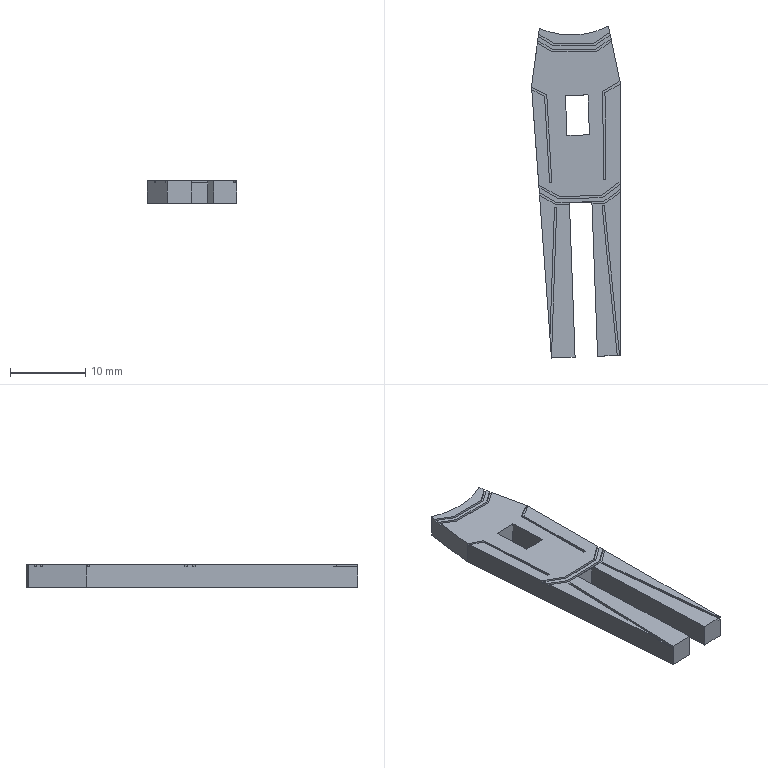Part | SolidWorks | features BaseBody 1 | 1 solid | 74 faces | box 11.853 x 44.2 x 3 mm | volume 1124 mm3 | plane 67 | spline 7